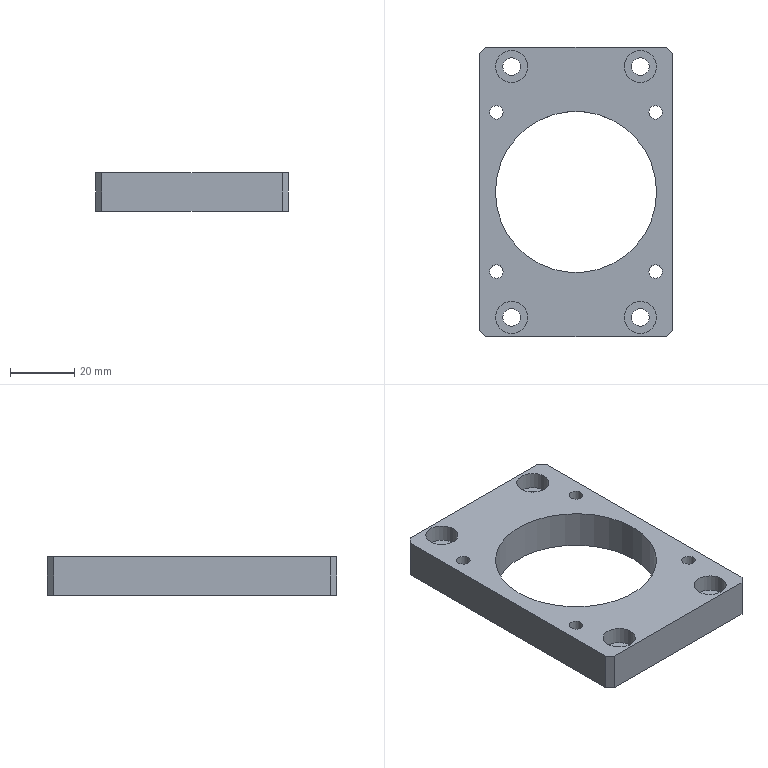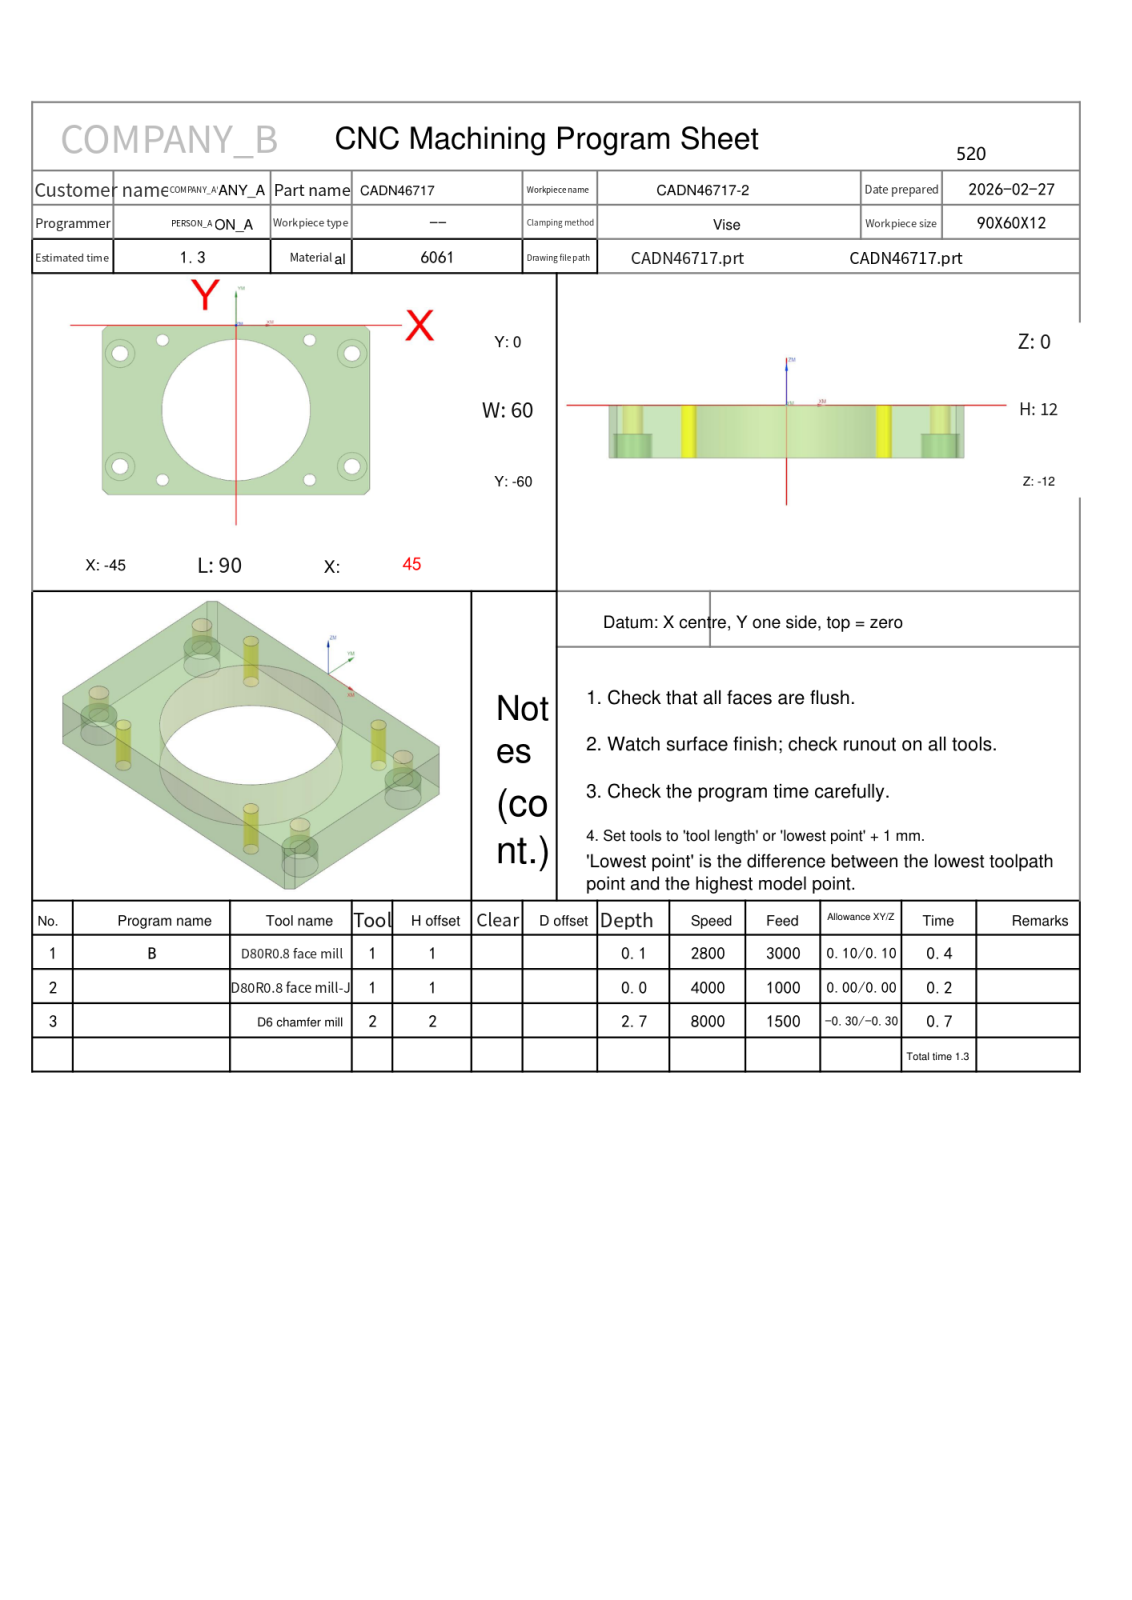NC program | NX | posted by the shop | part box 60 x 90 x 12 mm
Whole program:
%
O0001
(Machine time: 1.91 MIN)
(===Total Tool:2===)
(T1=D80R0.8 face mill D=80.  R=0.8  D-  H01 Z=-0.   )
(T2=D6 chamfer mill   D=6.   R=0.   D-  H02 Z=-2.7  )
G80 G90 G17 G49 G40
G91 G28 Z0
M01
N1 T01 M06
(D80R0.8 face mill D=80. R=0.8 H=01 ce=0.10 di=0.10)
G00 G90 G54 X-97.097 Y-30. M03 S2800
G43 H01 Z50.
M08
Z4.02
G01 Z2.02 F3000.
X-85.097
X85.097
X97.097
Z4.02
G00 X-97.097
Z3.54
G01 Z1.54
X-85.097
X85.097
X97.097
Z3.54
G00 X-97.097
Z3.06
G01 Z1.06
X-85.097
X85.097
X97.097
Z3.06
G00 X-97.097
Z2.58
G01 Z.58
X-85.097
X85.097
X97.097
Z2.58
G00 Z50.
X-97.097
Z2.1
G01 Z.1
X-85.097
X85.097
X97.097
Z2.1
G00 Z50.
G91 G28 Z0.0
M05
M09
G91 G28 Z0.0
M01
N2 T01 M06
(D80R0.8 face mill-J  D=80. R=0.8 H=01 ce=0.00 di=0.00)
G00 G90 G54 X-96.999 Y-30. M03 S4000
G43 H01 Z50.
M08
Z2.
G01 Z0.0 F1000.
X-84.999
X84.999
X96.999
Z2.
G00 Z50.
G91 G28 Z0.0
M05
M09
G91 G28 Z0.0
M01
N3 T02 M06
(D6 chamfer mill  D=6. R=0. H=02 ce=-0.30 di=0.00)
G00 G90 G54 X9.367 Y-7.526 M03 S7000
G43 H02 Z50.
M08
Z2.5
G01 X8.735 Y-7.267 Z2.251 F1500.
X7.729 Y-6.906 Z1.862
X6.708 Y-6.589 Z1.473
X5.674 Y-6.317 Z1.084
X4.63 Y-6.091 Z.695
X3.576 Y-5.911 Z.306
X2.516 Y-5.777 Z-.083
X1.45 Y-5.69 Z-.472
X.382 Y-5.65 Z-.861
X0.0 Z-1.
G03 X-24.35 Y-30. I0.0 J-24.35
X0.0 Y-54.35 I24.35 J0.0
X24.35 Y-30. I0.0 J24.35
X0.0 Y-5.65 I-24.35 J0.0
X-.5 Y-5.655 I0.0 J-24.35
G01 Z1.5
G00 Z50.
G00 G90 X24.749 Y-54.749 M03 S8000
Z50.
G98 G81 X24.749 Y-54.749 Z-2.7 R3. F1000.
Y-5.251
X-24.749
Y-54.749
G80
G00 Z50.
G00 G90 X38.353 Y-10.065 M03 S8000
Z50.
Z-.9
G01 Z-1.4 F1200.
X37.5 Y-10.15
G03 X39. Y-11.65 I1.5 J0.0
X40.65 Y-10. I0.0 J1.65
X39. Y-8.35 I-1.65 J0.0
X37.35 Y-10. I0.0 J-1.65
X39. Y-11.65 I1.65 J0.0
X40.5 Y-10.15 I0.0 J1.5
G01 X39.647 Y-10.065
Z-.9
G00 Z50.
X38.353 Y-50.065
Z-.9
G01 Z-1.4
X37.5 Y-50.15
G03 X39. Y-51.65 I1.5 J0.0
X40.65 Y-50. I0.0 J1.65
X39. Y-48.35 I-1.65 J0.0
X37.35 Y-50. I0.0 J-1.65
X39. Y-51.65 I1.65 J0.0
X40.5 Y-50.15 I0.0 J1.5
G01 X39.647 Y-50.065
Z-.9
G00 Z50.
X-39.647
Z-.9
G01 Z-1.4
X-40.5 Y-50.15
G03 X-39. Y-51.65 I1.5 J0.0
X-37.35 Y-50. I0.0 J1.65
X-39. Y-48.35 I-1.65 J0.0
X-40.65 Y-50. I0.0 J-1.65
X-39. Y-51.65 I1.65 J0.0
X-37.5 Y-50.15 I0.0 J1.5
G01 X-38.353 Y-50.065
Z-.9
G00 Z50.
X-39.647 Y-10.065
Z-.9
G01 Z-1.4
X-40.5 Y-10.15
G03 X-39. Y-11.65 I1.5 J0.0
X-37.35 Y-10. I0.0 J1.65
X-39. Y-8.35 I-1.65 J0.0
X-40.65 Y-10. I0.0 J-1.65
X-39. Y-11.65 I1.65 J0.0
X-37.5 Y-10.15 I0.0 J1.5
G01 X-38.353 Y-10.065
Z-.9
G00 Z50.
G00 G90 X.386 Y-61.227 M03 S6500
Z50.
Z.172
G01 Z-1.2 F1500.
G03 X.1 Y-61.027 I-1.286 J-1.532
G01 X.054 Y-60.997
X0.0 Y-61.
X-43.
X-43.259 Y-60.966
X-43.5 Y-60.866
X-43.707 Y-60.707
X-45.707 Y-58.707
X-45.866 Y-58.5
X-45.966 Y-58.259
X-46. Y-58.
Y-2.
X-45.966 Y-1.741
X-45.866 Y-1.5
X-45.707 Y-1.293
X-43.707 Y.707
X-43.5 Y.866
X-43.259 Y.966
X-43. Y1.
X43.
X43.259 Y.966
X43.5 Y.866
X43.707 Y.707
X45.707 Y-1.293
X45.866 Y-1.5
X45.966 Y-1.741
X46. Y-2.
Y-58.
X45.966 Y-58.259
X45.866 Y-58.5
X45.707 Y-58.707
X43.707 Y-60.707
X43.5 Y-60.866
X43.259 Y-60.966
X43. Y-61.
X0.0
X-.054 Y-60.997
X-.1 Y-61.027
G03 X-.386 Y-61.227 I1. J-1.732
G01 Z.172
G00 Z10.
X38.593 Y-51.565
Z.27
G01 Z-1.2
G03 X38.898 Y-51.734 I1.118 J1.658
G01 X38.946 Y-51.759
X39. Y-51.75
G03 X40.75 Y-50. I0.0 J1.75
X39. Y-48.25 I-1.75 J0.0
X37.25 Y-50. I0.0 J-1.75
X39. Y-51.75 I1.75 J0.0
G01 X39.054 Y-51.759
X39.102 Y-51.734
G03 X39.407 Y-51.565 I-.813 J1.827
G01 Z.27
G00 Z10.
X24.337 Y-55.674
Z.32
G01 Z-1.2
G03 X24.646 Y-55.835 I1.075 J1.687
G01 X24.695 Y-55.859
X24.749 Y-55.849
G03 X25.849 Y-54.749 I0.0 J1.1
X24.749 Y-53.649 I-1.1 J0.0
X23.649 Y-54.749 I0.0 J-1.1
X24.749 Y-55.849 I1.1 J0.0
G01 X24.802 Y-55.859
X24.851 Y-55.835
G03 X25.161 Y-55.674 I-.765 J1.848
G01 Z.32
G00 Z10.
X38.593 Y-11.565
Z.27
G01 Z-1.2
G03 X38.898 Y-11.734 I1.118 J1.658
G01 X38.946 Y-11.759
X39. Y-11.75
G03 X40.75 Y-10. I0.0 J1.75
X39. Y-8.25 I-1.75 J0.0
X37.25 Y-10. I0.0 J-1.75
X39. Y-11.75 I1.75 J0.0
G01 X39.054 Y-11.759
X39.102 Y-11.734
G03 X39.407 Y-11.565 I-.813 J1.827
G01 Z.27
G00 Z10.
X24.337 Y-6.177
Z.32
G01 Z-1.2
G03 X24.646 Y-6.338 I1.075 J1.687
G01 X24.695 Y-6.361
X24.749 Y-6.351
G03 X25.849 Y-5.251 I0.0 J1.1
X24.749 Y-4.151 I-1.1 J0.0
X23.649 Y-5.251 I0.0 J-1.1
X24.749 Y-6.351 I1.1 J0.0
G01 X24.802 Y-6.361
X24.851 Y-6.338
G03 X25.161 Y-6.177 I-.765 J1.848
G01 Z.32
G00 Z10.
X-.392 Y-53.834
Z.194
G01 Z-1.2
G03 X-.101 Y-54.026 I1.243 J1.567
G01 X-.054 Y-54.054
X0.0 Y-54.05
G03 X24.05 Y-30. I0.0 J24.05
X0.0 Y-5.95 I-24.05 J0.0
X-24.05 Y-30. I0.0 J-24.05
X0.0 Y-54.05 I24.05 J0.0
G01 X.054 Y-54.054
X.101 Y-54.026
G03 X.392 Y-53.834 I-.952 J1.759
G01 Z.194
G00 Z10.
X-25.161 Y-6.177
Z.32
G01 Z-1.2
G03 X-24.851 Y-6.338 I1.075 J1.687
G01 X-24.802 Y-6.361
X-24.749 Y-6.351
G03 X-23.649 Y-5.251 I0.0 J1.1
X-24.749 Y-4.151 I-1.1 J0.0
X-25.849 Y-5.251 I0.0 J-1.1
X-24.749 Y-6.351 I1.1 J0.0
G01 X-24.695 Y-6.361
X-24.646 Y-6.338
G03 X-24.337 Y-6.177 I-.765 J1.848
G01 Z.32
G00 Z10.
X-39.407 Y-11.565
Z.27
G01 Z-1.2
G03 X-39.102 Y-11.734 I1.118 J1.658
G01 X-39.054 Y-11.759
X-39. Y-11.75
G03 X-37.25 Y-10. I0.0 J1.75
X-39. Y-8.25 I-1.75 J0.0
X-40.75 Y-10. I0.0 J-1.75
X-39. Y-11.75 I1.75 J0.0
G01 X-38.946 Y-11.759
X-38.898 Y-11.734
G03 X-38.593 Y-11.565 I-.813 J1.827
G01 Z.27
G00 Z10.
X-39.407 Y-51.565
Z.27
G01 Z-1.2
G03 X-39.102 Y-51.734 I1.118 J1.658
G01 X-39.054 Y-51.759
X-39. Y-51.75
G03 X-37.25 Y-50. I0.0 J1.75
X-39. Y-48.25 I-1.75 J0.0
X-40.75 Y-50. I0.0 J-1.75
X-39. Y-51.75 I1.75 J0.0
G01 X-38.946 Y-51.759
X-38.898 Y-51.734
G03 X-38.593 Y-51.565 I-.813 J1.827
G01 Z.27
G00 Z10.
X-25.161 Y-55.674
Z.32
G01 Z-1.2
G03 X-24.851 Y-55.835 I1.075 J1.687
G01 X-24.802 Y-55.859
X-24.749 Y-55.849
G03 X-23.649 Y-54.749 I0.0 J1.1
X-24.749 Y-53.649 I-1.1 J0.0
X-25.849 Y-54.749 I0.0 J-1.1
X-24.749 Y-55.849 I1.1 J0.0
G01 X-24.695 Y-55.859
X-24.646 Y-55.835
G03 X-24.337 Y-55.674 I-.765 J1.848
G01 Z.32
G00 Z50.
M05
M09
G91 G28 Z0.0
G91 G28 Y0.0
M30
%